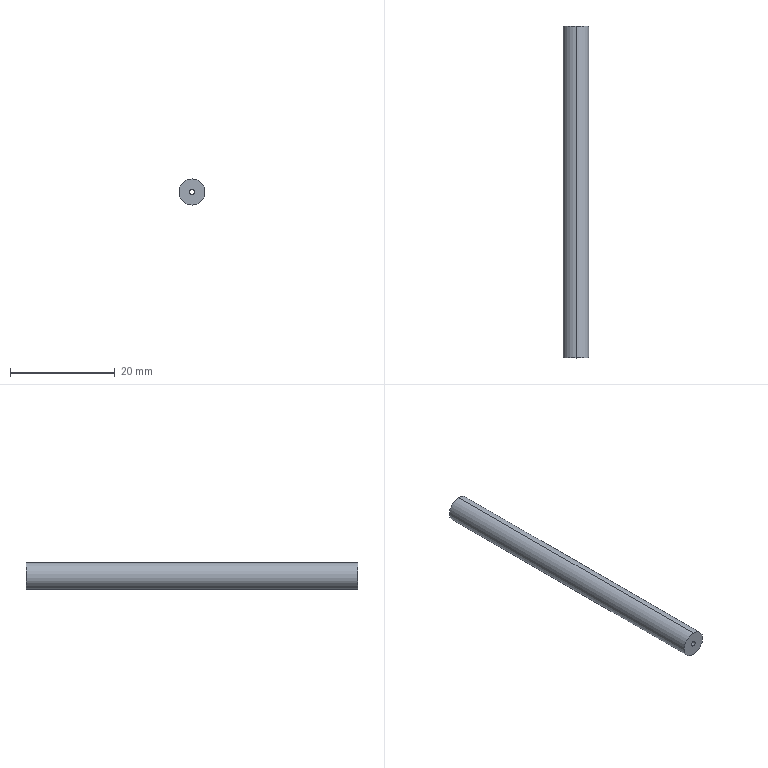Part | SolidWorks | features Extrusion 1, ICE 1 | 1 solid | 9 faces | box 5 x 63.5 x 5 mm | volume 810.531 mm3 | cylinder 6 | plane 3 | commonest cylinder face diameters 1 x2 3 x2 5 x2
STEP:
#1=CARTESIAN_POINT('',(0.,2.,0.5));
#2=VERTEX_POINT('',#1);
#3=CARTESIAN_POINT('',(0.,2.,-0.5));
#4=VERTEX_POINT('',#3);
#5=CARTESIAN_POINT('',(0.,2.,0.));
#6=DIRECTION('',(0.,-1.,0.));
#7=DIRECTION('',(0.,0.,-1.));
#8=AXIS2_PLACEMENT_3D('',#5,#6,#7);
#9=CIRCLE('',#8,0.5);
#10=EDGE_CURVE('',#2,#4,#9,.T.);
#11=ORIENTED_EDGE('',*,*,#10,.F.);
#12=CARTESIAN_POINT('',(0.,0.,0.5));
#13=VERTEX_POINT('',#12);
#14=CARTESIAN_POINT('',(0.,2.,0.5));
#15=DIRECTION('',(0.,-1.,0.));
#16=VECTOR('',#15,1000.);
#17=LINE('',#14,#16);
#18=EDGE_CURVE('',#2,#13,#17,.T.);
#19=ORIENTED_EDGE('',*,*,#18,.T.);
#20=CARTESIAN_POINT('',(0.,0.,-0.5));
#21=VERTEX_POINT('',#20);
#22=CARTESIAN_POINT('',(0.,0.,0.));
#23=DIRECTION('',(0.,-1.,0.));
#24=DIRECTION('',(0.,0.,-1.));
#25=AXIS2_PLACEMENT_3D('',#22,#23,#24);
#26=CIRCLE('',#25,0.5);
#27=EDGE_CURVE('',#13,#21,#26,.T.);
#28=ORIENTED_EDGE('',*,*,#27,.T.);
#29=CARTESIAN_POINT('',(0.,2.,-0.5));
#30=DIRECTION('',(0.,-1.,0.));
#31=VECTOR('',#30,1000.);
#32=LINE('',#29,#31);
#33=EDGE_CURVE('',#4,#21,#32,.T.);
#34=ORIENTED_EDGE('',*,*,#33,.F.);
#35=EDGE_LOOP('',(#11,#19,#28,#34));
#36=FACE_OUTER_BOUND('',#35,.T.);
#37=CARTESIAN_POINT('',(0.,2.,0.));
#38=DIRECTION('',(0.,-1.,0.));
#39=DIRECTION('',(0.,0.,-1.));
#40=AXIS2_PLACEMENT_3D('',#37,#38,#39);
#41=CYLINDRICAL_SURFACE('',#40,0.5);
#42=ADVANCED_FACE('',(#36),#41,.F.);
#43=CARTESIAN_POINT('',(0.,63.5,2.5));
#44=VERTEX_POINT('',#43);
#45=CARTESIAN_POINT('',(0.,63.5,-2.5));
#46=VERTEX_POINT('',#45);
#47=CARTESIAN_POINT('',(0.,63.5,0.));
#48=DIRECTION('',(0.,1.,0.));
#49=DIRECTION('',(0.,0.,1.));
#50=AXIS2_PLACEMENT_3D('',#47,#48,#49);
#51=CIRCLE('',#50,2.5);
#52=EDGE_CURVE('',#44,#46,#51,.T.);
#53=ORIENTED_EDGE('',*,*,#52,.F.);
#54=CARTESIAN_POINT('',(0.,0.,2.5));
#55=VERTEX_POINT('',#54);
#56=CARTESIAN_POINT('',(0.,63.5,2.5));
#57=DIRECTION('',(0.,-1.,0.));
#58=VECTOR('',#57,1000.);
#59=LINE('',#56,#58);
#60=EDGE_CURVE('',#44,#55,#59,.T.);
#61=ORIENTED_EDGE('',*,*,#60,.T.);
#62=CARTESIAN_POINT('',(0.,0.,-2.5));
#63=VERTEX_POINT('',#62);
#64=CARTESIAN_POINT('',(0.,0.,0.));
#65=DIRECTION('',(0.,1.,0.));
#66=DIRECTION('',(0.,0.,1.));
#67=AXIS2_PLACEMENT_3D('',#64,#65,#66);
#68=CIRCLE('',#67,2.5);
#69=EDGE_CURVE('',#55,#63,#68,.T.);
#70=ORIENTED_EDGE('',*,*,#69,.T.);
#71=CARTESIAN_POINT('',(0.,63.5,-2.5));
#72=DIRECTION('',(0.,-1.,0.));
#73=VECTOR('',#72,1000.);
#74=LINE('',#71,#73);
#75=EDGE_CURVE('',#46,#63,#74,.T.);
#76=ORIENTED_EDGE('',*,*,#75,.F.);
#77=EDGE_LOOP('',(#53,#61,#70,#76));
#78=FACE_OUTER_BOUND('',#77,.T.);
#79=CARTESIAN_POINT('',(0.,63.5,0.));
#80=DIRECTION('',(0.,-1.,0.));
#81=DIRECTION('',(0.,0.,-1.));
#82=AXIS2_PLACEMENT_3D('',#79,#80,#81);
#83=CYLINDRICAL_SURFACE('',#82,2.5);
#84=ADVANCED_FACE('',(#78),#83,.T.);
#85=CARTESIAN_POINT('',(0.,63.5,-1.5));
#86=VERTEX_POINT('',#85);
#87=CARTESIAN_POINT('',(0.,63.5,1.5));
#88=VERTEX_POINT('',#87);
#89=CARTESIAN_POINT('',(0.,63.5,0.));
#90=DIRECTION('',(0.,1.,0.));
#91=DIRECTION('',(0.,0.,1.));
#92=AXIS2_PLACEMENT_3D('',#89,#90,#91);
#93=CIRCLE('',#92,1.5);
#94=EDGE_CURVE('',#86,#88,#93,.T.);
#95=ORIENTED_EDGE('',*,*,#94,.T.);
#96=CARTESIAN_POINT('',(0.,2.,1.5));
#97=VERTEX_POINT('',#96);
#98=CARTESIAN_POINT('',(0.,63.5,1.5));
#99=DIRECTION('',(0.,-1.,0.));
#100=VECTOR('',#99,1000.);
#101=LINE('',#98,#100);
#102=EDGE_CURVE('',#88,#97,#101,.T.);
#103=ORIENTED_EDGE('',*,*,#102,.T.);
#104=CARTESIAN_POINT('',(0.,2.,-1.5));
#105=VERTEX_POINT('',#104);
#106=CARTESIAN_POINT('',(0.,2.,0.));
#107=DIRECTION('',(0.,-1.,0.));
#108=DIRECTION('',(0.,0.,-1.));
#109=AXIS2_PLACEMENT_3D('',#106,#107,#108);
#110=CIRCLE('',#109,1.5);
#111=EDGE_CURVE('',#97,#105,#110,.T.);
#112=ORIENTED_EDGE('',*,*,#111,.T.);
#113=CARTESIAN_POINT('',(0.,63.5,-1.5));
#114=DIRECTION('',(0.,-1.,0.));
#115=VECTOR('',#114,1000.);
#116=LINE('',#113,#115);
#117=EDGE_CURVE('',#86,#105,#116,.T.);
#118=ORIENTED_EDGE('',*,*,#117,.F.);
#119=EDGE_LOOP('',(#95,#103,#112,#118));
#120=FACE_OUTER_BOUND('',#119,.T.);
#121=CARTESIAN_POINT('',(0.,63.5,0.));
#122=DIRECTION('',(0.,-1.,0.));
#123=DIRECTION('',(0.,0.,-1.));
#124=AXIS2_PLACEMENT_3D('',#121,#122,#123);
#125=CYLINDRICAL_SURFACE('',#124,1.5);
#126=ADVANCED_FACE('',(#120),#125,.F.);
#127=ORIENTED_EDGE('',*,*,#102,.F.);
#128=CARTESIAN_POINT('',(0.,63.5,0.));
#129=DIRECTION('',(0.,1.,0.));
#130=DIRECTION('',(0.,0.,1.));
#131=AXIS2_PLACEMENT_3D('',#128,#129,#130);
#132=CIRCLE('',#131,1.5);
#133=EDGE_CURVE('',#88,#86,#132,.T.);
#134=ORIENTED_EDGE('',*,*,#133,.T.);
#135=ORIENTED_EDGE('',*,*,#117,.T.);
#136=CARTESIAN_POINT('',(0.,2.,0.));
#137=DIRECTION('',(0.,-1.,0.));
#138=DIRECTION('',(0.,0.,-1.));
#139=AXIS2_PLACEMENT_3D('',#136,#137,#138);
#140=CIRCLE('',#139,1.5);
#141=EDGE_CURVE('',#105,#97,#140,.T.);
#142=ORIENTED_EDGE('',*,*,#141,.T.);
#143=EDGE_LOOP('',(#127,#134,#135,#142));
#144=FACE_OUTER_BOUND('',#143,.T.);
#145=CARTESIAN_POINT('',(0.,63.5,0.));
#146=DIRECTION('',(0.,-1.,0.));
#147=DIRECTION('',(0.,0.,-1.));
#148=AXIS2_PLACEMENT_3D('',#145,#146,#147);
#149=CYLINDRICAL_SURFACE('',#148,1.5);
#150=ADVANCED_FACE('',(#144),#149,.F.);
#151=CARTESIAN_POINT('',(0.,63.5,0.));
#152=DIRECTION('',(0.,1.,0.));
#153=DIRECTION('',(0.,0.,1.));
#154=AXIS2_PLACEMENT_3D('',#151,#152,#153);
#155=CIRCLE('',#154,2.5);
#156=EDGE_CURVE('',#46,#44,#155,.T.);
#157=ORIENTED_EDGE('',*,*,#156,.T.);
#158=ORIENTED_EDGE('',*,*,#52,.T.);
#159=EDGE_LOOP('',(#157,#158));
#160=FACE_OUTER_BOUND('',#159,.T.);
#161=ORIENTED_EDGE('',*,*,#94,.F.);
#162=ORIENTED_EDGE('',*,*,#133,.F.);
#163=EDGE_LOOP('',(#161,#162));
#164=FACE_BOUND('',#163,.T.);
#165=CARTESIAN_POINT('',(0.,63.5,0.));
#166=DIRECTION('',(0.,1.,0.));
#167=DIRECTION('',(0.,0.,1.));
#168=AXIS2_PLACEMENT_3D('',#165,#166,#167);
#169=PLANE('',#168);
#170=ADVANCED_FACE('',(#160,#164),#169,.T.);
#171=CARTESIAN_POINT('',(0.,0.,0.));
#172=DIRECTION('',(0.,1.,0.));
#173=DIRECTION('',(0.,0.,1.));
#174=AXIS2_PLACEMENT_3D('',#171,#172,#173);
#175=CIRCLE('',#174,2.5);
#176=EDGE_CURVE('',#63,#55,#175,.T.);
#177=ORIENTED_EDGE('',*,*,#176,.F.);
#178=ORIENTED_EDGE('',*,*,#69,.F.);
#179=EDGE_LOOP('',(#177,#178));
#180=FACE_OUTER_BOUND('',#179,.T.);
#181=CARTESIAN_POINT('',(0.,0.,0.));
#182=DIRECTION('',(0.,-1.,0.));
#183=DIRECTION('',(0.,0.,-1.));
#184=AXIS2_PLACEMENT_3D('',#181,#182,#183);
#185=CIRCLE('',#184,0.5);
#186=EDGE_CURVE('',#21,#13,#185,.T.);
#187=ORIENTED_EDGE('',*,*,#186,.F.);
#188=ORIENTED_EDGE('',*,*,#27,.F.);
#189=EDGE_LOOP('',(#187,#188));
#190=FACE_BOUND('',#189,.T.);
#191=CARTESIAN_POINT('',(0.,0.,0.));
#192=DIRECTION('',(0.,1.,0.));
#193=DIRECTION('',(0.,0.,1.));
#194=AXIS2_PLACEMENT_3D('',#191,#192,#193);
#195=PLANE('',#194);
#196=ADVANCED_FACE('',(#180,#190),#195,.F.);
#197=ORIENTED_EDGE('',*,*,#60,.F.);
#198=ORIENTED_EDGE('',*,*,#156,.F.);
#199=ORIENTED_EDGE('',*,*,#75,.T.);
#200=ORIENTED_EDGE('',*,*,#176,.T.);
#201=EDGE_LOOP('',(#197,#198,#199,#200));
#202=FACE_OUTER_BOUND('',#201,.T.);
#203=CARTESIAN_POINT('',(0.,63.5,0.));
#204=DIRECTION('',(0.,-1.,0.));
#205=DIRECTION('',(0.,0.,-1.));
#206=AXIS2_PLACEMENT_3D('',#203,#204,#205);
#207=CYLINDRICAL_SURFACE('',#206,2.5);
#208=ADVANCED_FACE('',(#202),#207,.T.);
#209=CARTESIAN_POINT('',(0.,2.,0.));
#210=DIRECTION('',(0.,-1.,0.));
#211=DIRECTION('',(0.,0.,-1.));
#212=AXIS2_PLACEMENT_3D('',#209,#210,#211);
#213=CIRCLE('',#212,0.5);
#214=EDGE_CURVE('',#4,#2,#213,.T.);
#215=ORIENTED_EDGE('',*,*,#214,.T.);
#216=ORIENTED_EDGE('',*,*,#10,.T.);
#217=EDGE_LOOP('',(#215,#216));
#218=FACE_BOUND('',#217,.T.);
#219=ORIENTED_EDGE('',*,*,#141,.F.);
#220=ORIENTED_EDGE('',*,*,#111,.F.);
#221=EDGE_LOOP('',(#219,#220));
#222=FACE_OUTER_BOUND('',#221,.T.);
#223=CARTESIAN_POINT('',(0.,2.,0.));
#224=DIRECTION('',(0.,-1.,0.));
#225=DIRECTION('',(0.,0.,-1.));
#226=AXIS2_PLACEMENT_3D('',#223,#224,#225);
#227=PLANE('',#226);
#228=ADVANCED_FACE('',(#218,#222),#227,.F.);
#229=ORIENTED_EDGE('',*,*,#18,.F.);
#230=ORIENTED_EDGE('',*,*,#214,.F.);
#231=ORIENTED_EDGE('',*,*,#33,.T.);
#232=ORIENTED_EDGE('',*,*,#186,.T.);
#233=EDGE_LOOP('',(#229,#230,#231,#232));
#234=FACE_OUTER_BOUND('',#233,.T.);
#235=CARTESIAN_POINT('',(0.,2.,0.));
#236=DIRECTION('',(0.,-1.,0.));
#237=DIRECTION('',(0.,0.,-1.));
#238=AXIS2_PLACEMENT_3D('',#235,#236,#237);
#239=CYLINDRICAL_SURFACE('',#238,0.5);
#240=ADVANCED_FACE('',(#234),#239,.F.);
#241=CLOSED_SHELL('',(#42,#84,#126,#150,#170,#196,#208,#228,#240));
#242=MANIFOLD_SOLID_BREP('',#241);
#243=CARTESIAN_POINT('',(0.,0.,0.));
#244=DIRECTION('',(0.,0.,1.));
#245=DIRECTION('',(1.,0.,0.));
#246=AXIS2_PLACEMENT_3D('',#243,#244,#245);
#247=(LENGTH_UNIT()NAMED_UNIT(*)SI_UNIT(.MILLI.,.METRE.));
#248=UNCERTAINTY_MEASURE_WITH_UNIT(LENGTH_MEASURE(0.00001),#247,'','');
#249=(NAMED_UNIT(*)PLANE_ANGLE_UNIT()SI_UNIT($,.RADIAN.));
#250=(NAMED_UNIT(*)SI_UNIT($,.STERADIAN.)SOLID_ANGLE_UNIT());
#251=(GEOMETRIC_REPRESENTATION_CONTEXT(3)GLOBAL_UNCERTAINTY_ASSIGNED_CONTEXT((#248))GLOBAL_UNIT_ASSIGNED_CONTEXT((#247,#249,#250))REPRESENTATION_CONTEXT('',''));
#252=ADVANCED_BREP_SHAPE_REPRESENTATION('',(#242,#246),#251);